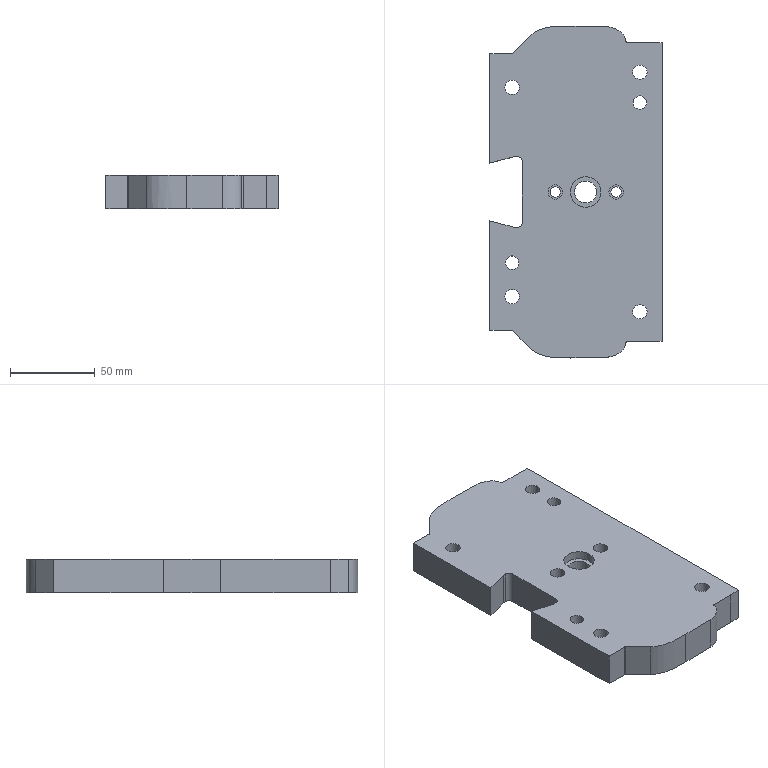Part | NX | features solid 2 | 1 solid | 57 faces | box 101.709 x 196.21 x 20 mm | volume 344496 mm3 | plane 25 | cylinder 22 | spline 10 | commonest cylinder face diameters 8.5 x8 14 x4 2 x2 6 x2 6.1 x2 8 x2